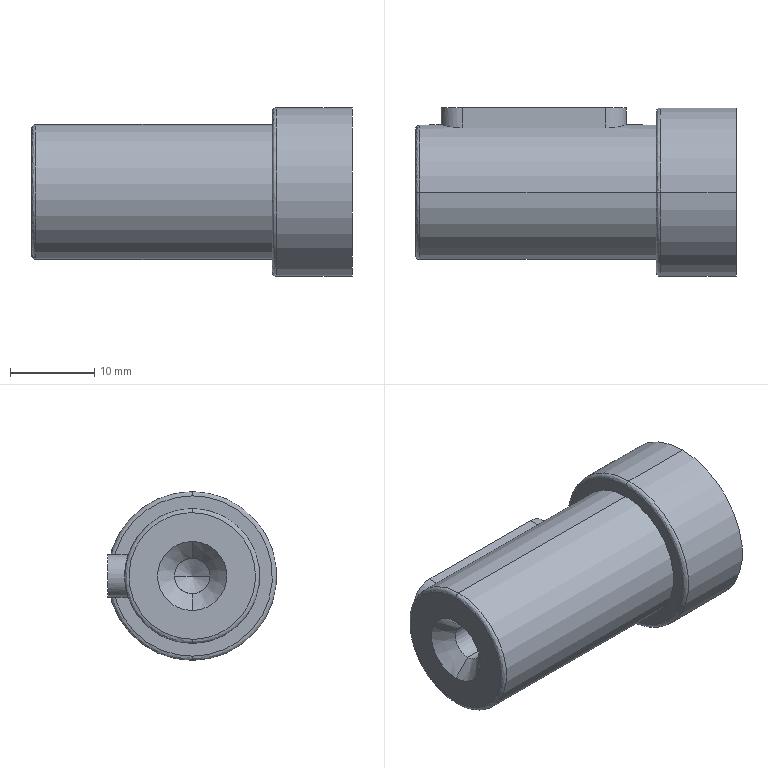Part | STEP file | _X2_8f9351fa884c661f67b6_X0_MAB060-16X28.5XM5_2.STEP.STEP | 1 solid | 22 faces | box 38 x 20 x 20 mm | volume 8651 mm3 | cylinder 8 | plane 6 | spline 4 | cone 4 | commonest cylinder face diameters 4.2 x2 5 x2 16 x2 20 x2
STEP:
#1=CARTESIAN_POINT('',(9.288,0.,7.5));
#2=VERTEX_POINT('',#1);
#3=CARTESIAN_POINT('',(9.288,0.,-7.5));
#4=VERTEX_POINT('',#3);
#5=CARTESIAN_POINT('',(9.288,0.,7.5));
#6=CARTESIAN_POINT('',(9.288,-15.,7.5));
#7=CARTESIAN_POINT('',(9.288,-15.,-7.5));
#8=CARTESIAN_POINT('',(9.288,0.,-7.5));
#9=(BOUNDED_CURVE()B_SPLINE_CURVE(3,(#5,#6,#7,#8),.UNSPECIFIED.,.F.,.F.)B_SPLINE_CURVE_WITH_KNOTS((4,4),(0.,1.),.UNSPECIFIED.)CURVE()GEOMETRIC_REPRESENTATION_ITEM()RATIONAL_B_SPLINE_CURVE((1.,0.3333,0.3333,1.))REPRESENTATION_ITEM(''));
#10=EDGE_CURVE('',#2,#4,#9,.T.);
#11=ORIENTED_EDGE('',*,*,#10,.T.);
#12=CARTESIAN_POINT('',(9.788,0.,-8.));
#13=VERTEX_POINT('',#12);
#14=CARTESIAN_POINT('',(9.788,0.,-7.5));
#15=DIRECTION('',(0.,-1.,0.));
#16=DIRECTION('',(0.,0.,-1.));
#17=AXIS2_PLACEMENT_3D('',#14,#15,#16);
#18=CIRCLE('',#17,0.5);
#19=EDGE_CURVE('',#4,#13,#18,.T.);
#20=ORIENTED_EDGE('',*,*,#19,.T.);
#21=CARTESIAN_POINT('',(9.788,0.,8.));
#22=VERTEX_POINT('',#21);
#23=CARTESIAN_POINT('',(9.788,0.,0.));
#24=DIRECTION('',(1.,0.,0.));
#25=DIRECTION('',(0.,0.,-1.));
#26=AXIS2_PLACEMENT_3D('',#23,#24,#25);
#27=CIRCLE('',#26,8.);
#28=EDGE_CURVE('',#22,#13,#27,.T.);
#29=ORIENTED_EDGE('',*,*,#28,.F.);
#30=CARTESIAN_POINT('',(9.788,0.,7.5));
#31=DIRECTION('',(0.,1.,0.));
#32=DIRECTION('',(0.,0.,1.));
#33=AXIS2_PLACEMENT_3D('',#30,#31,#32);
#34=CIRCLE('',#33,0.5);
#35=EDGE_CURVE('',#2,#22,#34,.T.);
#36=ORIENTED_EDGE('',*,*,#35,.F.);
#37=EDGE_LOOP('',(#11,#20,#29,#36));
#38=FACE_OUTER_BOUND('',#37,.T.);
#39=CARTESIAN_POINT('',(9.288,0.,-7.5));
#40=CARTESIAN_POINT('',(9.288,-15.,-7.5));
#41=CARTESIAN_POINT('',(9.288,-15.,7.5));
#42=CARTESIAN_POINT('',(9.288,0.,7.5));
#43=CARTESIAN_POINT('',(9.288,0.,-7.793));
#44=CARTESIAN_POINT('',(9.288,-15.586,-7.793));
#45=CARTESIAN_POINT('',(9.288,-15.586,7.793));
#46=CARTESIAN_POINT('',(9.288,0.,7.793));
#47=CARTESIAN_POINT('',(9.495,0.,-8.));
#48=CARTESIAN_POINT('',(9.495,-16.,-8.));
#49=CARTESIAN_POINT('',(9.495,-16.,8.));
#50=CARTESIAN_POINT('',(9.495,0.,8.));
#51=CARTESIAN_POINT('',(9.788,0.,-8.));
#52=CARTESIAN_POINT('',(9.788,-16.,-8.));
#53=CARTESIAN_POINT('',(9.788,-16.,8.));
#54=CARTESIAN_POINT('',(9.788,0.,8.));
#55=(BOUNDED_SURFACE()B_SPLINE_SURFACE(3,3,((#39,#40,#41,#42),(#43,#44,#45,#46),(#47,#48,#49,#50),(#51,#52,#53,#54)),.UNSPECIFIED.,.F.,.F.,.T.)B_SPLINE_SURFACE_WITH_KNOTS((4,4),(4,4),(0.,1.),(0.,1.),.UNSPECIFIED.)GEOMETRIC_REPRESENTATION_ITEM()RATIONAL_B_SPLINE_SURFACE(((1.,0.3333,0.3333,1.),(0.8047,0.2682,0.2682,0.8047),(0.8047,0.2682,0.2682,0.8047),(1.,0.3333,0.3333,1.)))REPRESENTATION_ITEM('')SURFACE());
#56=ADVANCED_FACE('',(#38),#55,.T.);
#57=CARTESIAN_POINT('',(37.788,0.,-9.5));
#58=VERTEX_POINT('',#57);
#59=CARTESIAN_POINT('',(37.788,0.,9.5));
#60=VERTEX_POINT('',#59);
#61=CARTESIAN_POINT('',(37.788,0.,-9.5));
#62=CARTESIAN_POINT('',(37.788,-0.2904,-9.5));
#63=CARTESIAN_POINT('',(37.788,-0.7244,-9.48));
#64=CARTESIAN_POINT('',(37.788,-1.228,-9.422));
#65=CARTESIAN_POINT('',(37.788,-1.478,-9.385));
#66=CARTESIAN_POINT('',(37.788,-1.586,-9.367));
#67=CARTESIAN_POINT('',(37.788,-1.657,-9.354));
#68=CARTESIAN_POINT('',(37.788,-1.691,-9.348));
#69=CARTESIAN_POINT('',(37.788,-2.031,-9.285));
#70=CARTESIAN_POINT('',(37.788,-2.48,-9.18));
#71=CARTESIAN_POINT('',(37.788,-2.992,-9.019));
#72=CARTESIAN_POINT('',(37.788,-3.245,-8.929));
#73=CARTESIAN_POINT('',(37.788,-3.353,-8.889));
#74=CARTESIAN_POINT('',(37.788,-3.425,-8.861));
#75=CARTESIAN_POINT('',(37.788,-3.46,-8.848));
#76=CARTESIAN_POINT('',(37.788,-3.795,-8.715));
#77=CARTESIAN_POINT('',(37.788,-4.232,-8.516));
#78=CARTESIAN_POINT('',(37.788,-4.722,-8.246));
#79=CARTESIAN_POINT('',(37.788,-4.927,-8.123));
#80=CARTESIAN_POINT('',(37.788,-5.064,-8.038));
#81=CARTESIAN_POINT('',(37.788,-5.13,-7.996));
#82=CARTESIAN_POINT('',(37.788,-5.747,-7.593));
#83=CARTESIAN_POINT('',(37.788,-6.254,-7.181));
#84=CARTESIAN_POINT('',(37.788,-6.949,-6.486));
#85=CARTESIAN_POINT('',(37.788,-7.277,-6.122));
#86=CARTESIAN_POINT('',(37.788,-7.626,-5.67));
#87=CARTESIAN_POINT('',(37.788,-7.768,-5.47));
#88=CARTESIAN_POINT('',(37.788,-7.861,-5.335));
#89=CARTESIAN_POINT('',(37.788,-7.908,-5.266));
#90=CARTESIAN_POINT('',(37.788,-8.127,-4.93));
#91=CARTESIAN_POINT('',(37.788,-8.369,-4.516));
#92=CARTESIAN_POINT('',(37.788,-8.614,-4.013));
#93=CARTESIAN_POINT('',(37.788,-8.726,-3.757));
#94=CARTESIAN_POINT('',(37.788,-8.773,-3.646));
#95=CARTESIAN_POINT('',(37.788,-8.803,-3.571));
#96=CARTESIAN_POINT('',(37.788,-8.819,-3.533));
#97=CARTESIAN_POINT('',(37.788,-8.946,-3.211));
#98=CARTESIAN_POINT('',(37.788,-9.095,-2.775));
#99=CARTESIAN_POINT('',(37.788,-9.231,-2.255));
#100=CARTESIAN_POINT('',(37.788,-9.289,-1.993));
#101=CARTESIAN_POINT('',(37.788,-9.312,-1.88));
#102=CARTESIAN_POINT('',(37.788,-9.327,-1.804));
#103=CARTESIAN_POINT('',(37.788,-9.335,-1.764));
#104=CARTESIAN_POINT('',(37.788,-9.447,-1.158));
#105=CARTESIAN_POINT('',(37.788,-9.5,-0.5807));
#106=CARTESIAN_POINT('',(37.788,-9.5,0.2904));
#107=CARTESIAN_POINT('',(37.788,-9.48,0.7242));
#108=CARTESIAN_POINT('',(37.788,-9.422,1.227));
#109=CARTESIAN_POINT('',(37.788,-9.385,1.478));
#110=CARTESIAN_POINT('',(37.788,-9.367,1.586));
#111=CARTESIAN_POINT('',(37.788,-9.354,1.657));
#112=CARTESIAN_POINT('',(37.788,-9.348,1.691));
#113=CARTESIAN_POINT('',(37.788,-9.285,2.031));
#114=CARTESIAN_POINT('',(37.788,-9.18,2.48));
#115=CARTESIAN_POINT('',(37.788,-9.019,2.992));
#116=CARTESIAN_POINT('',(37.788,-8.929,3.245));
#117=CARTESIAN_POINT('',(37.788,-8.889,3.353));
#118=CARTESIAN_POINT('',(37.788,-8.861,3.425));
#119=CARTESIAN_POINT('',(37.788,-8.848,3.46));
#120=CARTESIAN_POINT('',(37.788,-8.715,3.795));
#121=CARTESIAN_POINT('',(37.788,-8.516,4.232));
#122=CARTESIAN_POINT('',(37.788,-8.246,4.722));
#123=CARTESIAN_POINT('',(37.788,-8.123,4.927));
#124=CARTESIAN_POINT('',(37.788,-8.038,5.064));
#125=CARTESIAN_POINT('',(37.788,-7.996,5.13));
#126=CARTESIAN_POINT('',(37.788,-7.593,5.747));
#127=CARTESIAN_POINT('',(37.788,-7.181,6.254));
#128=CARTESIAN_POINT('',(37.788,-6.486,6.949));
#129=CARTESIAN_POINT('',(37.788,-6.122,7.277));
#130=CARTESIAN_POINT('',(37.788,-5.67,7.626));
#131=CARTESIAN_POINT('',(37.788,-5.47,7.768));
#132=CARTESIAN_POINT('',(37.788,-5.335,7.861));
#133=CARTESIAN_POINT('',(37.788,-5.266,7.908));
#134=CARTESIAN_POINT('',(37.788,-4.93,8.127));
#135=CARTESIAN_POINT('',(37.788,-4.516,8.369));
#136=CARTESIAN_POINT('',(37.788,-4.013,8.614));
#137=CARTESIAN_POINT('',(37.788,-3.757,8.726));
#138=CARTESIAN_POINT('',(37.788,-3.646,8.773));
#139=CARTESIAN_POINT('',(37.788,-3.571,8.803));
#140=CARTESIAN_POINT('',(37.788,-3.533,8.819));
#141=CARTESIAN_POINT('',(37.788,-3.211,8.946));
#142=CARTESIAN_POINT('',(37.788,-2.775,9.095));
#143=CARTESIAN_POINT('',(37.788,-2.255,9.231));
#144=CARTESIAN_POINT('',(37.788,-1.993,9.289));
#145=CARTESIAN_POINT('',(37.788,-1.88,9.312));
#146=CARTESIAN_POINT('',(37.788,-1.804,9.327));
#147=CARTESIAN_POINT('',(37.788,-1.764,9.335));
#148=CARTESIAN_POINT('',(37.788,-1.157,9.447));
#149=CARTESIAN_POINT('',(37.788,-0.5812,9.5));
#150=CARTESIAN_POINT('',(37.788,0.,9.5));
#151=B_SPLINE_CURVE_WITH_KNOTS('',3,(#61,#62,#63,#64,#65,#66,#67,#68,#69,#70,#71,#72,#73,#74,#75,#76,#77,#78,#79,#80,#81,#82,#83,#84,#85,#86,#87,#88,#89,#90,#91,#92,#93,#94,#95,#96,#97,#98,#99,#100,#101,#102,#103,#104,#105,#106,#107,#108,#109,#110,#111,#112,#113,#114,#115,#116,#117,#118,#119,#120,#121,#122,#123,#124,#125,#126,#127,#128,#129,#130,#131,#132,#133,#134,#135,#136,#137,#138,#139,#140,#141,#142,#143,#144,#145,#146,#147,#148,#149,#150),.UNSPECIFIED.,.F.,.F.,(4,1,1,1,2,2,1,1,1,2,2,1,1,2,2,2,1,1,2,2,1,1,1,2,2,1,1,1,2,2,2,1,1,1,2,2,1,1,1,2,2,1,1,2,2,2,1,1,2,2,1,1,1,2,2,1,1,1,2,2,4),(0.,0.03125,0.04688,0.05469,0.05859,0.0625,0.09375,0.1094,0.1172,0.1211,0.125,0.1563,0.1719,0.1797,0.1875,0.25,0.2813,0.2969,0.3047,0.3125,0.3438,0.3594,0.3672,0.3711,0.375,0.4063,0.4219,0.4297,0.4336,0.4375,0.5,0.5313,0.5469,0.5547,0.5586,0.5625,0.5938,0.6094,0.6172,0.6211,0.625,0.6563,0.6719,0.6797,0.6875,0.75,0.7813,0.7969,0.8047,0.8125,0.8438,0.8594,0.8672,0.8711,0.875,0.9063,0.9219,0.9297,0.9336,0.9375,1.),.UNSPECIFIED.);
#152=EDGE_CURVE('',#58,#60,#151,.T.);
#153=ORIENTED_EDGE('',*,*,#152,.F.);
#154=CARTESIAN_POINT('',(38.288,0.,-10.));
#155=VERTEX_POINT('',#154);
#156=CARTESIAN_POINT('',(38.288,0.,-9.5));
#157=DIRECTION('',(0.,-1.,0.));
#158=DIRECTION('',(0.,0.,-1.));
#159=AXIS2_PLACEMENT_3D('',#156,#157,#158);
#160=CIRCLE('',#159,0.5);
#161=EDGE_CURVE('',#58,#155,#160,.T.);
#162=ORIENTED_EDGE('',*,*,#161,.T.);
#163=CARTESIAN_POINT('',(38.288,0.,10.));
#164=VERTEX_POINT('',#163);
#165=CARTESIAN_POINT('',(38.288,0.,0.));
#166=DIRECTION('',(-1.,0.,0.));
#167=DIRECTION('',(0.,0.,1.));
#168=AXIS2_PLACEMENT_3D('',#165,#166,#167);
#169=CIRCLE('',#168,10.);
#170=EDGE_CURVE('',#155,#164,#169,.T.);
#171=ORIENTED_EDGE('',*,*,#170,.T.);
#172=CARTESIAN_POINT('',(38.288,0.,9.5));
#173=DIRECTION('',(0.,1.,0.));
#174=DIRECTION('',(0.,0.,1.));
#175=AXIS2_PLACEMENT_3D('',#172,#173,#174);
#176=CIRCLE('',#175,0.5);
#177=EDGE_CURVE('',#60,#164,#176,.T.);
#178=ORIENTED_EDGE('',*,*,#177,.F.);
#179=EDGE_LOOP('',(#153,#162,#171,#178));
#180=FACE_OUTER_BOUND('',#179,.T.);
#181=CARTESIAN_POINT('',(37.788,0.,-9.5));
#182=CARTESIAN_POINT('',(37.788,-19.,-9.5));
#183=CARTESIAN_POINT('',(37.788,-19.,9.5));
#184=CARTESIAN_POINT('',(37.788,0.,9.5));
#185=CARTESIAN_POINT('',(37.788,0.,-9.793));
#186=CARTESIAN_POINT('',(37.788,-19.586,-9.793));
#187=CARTESIAN_POINT('',(37.788,-19.586,9.793));
#188=CARTESIAN_POINT('',(37.788,0.,9.793));
#189=CARTESIAN_POINT('',(37.995,0.,-10.));
#190=CARTESIAN_POINT('',(37.995,-20.,-10.));
#191=CARTESIAN_POINT('',(37.995,-20.,10.));
#192=CARTESIAN_POINT('',(37.995,0.,10.));
#193=CARTESIAN_POINT('',(38.288,0.,-10.));
#194=CARTESIAN_POINT('',(38.288,-20.,-10.));
#195=CARTESIAN_POINT('',(38.288,-20.,10.));
#196=CARTESIAN_POINT('',(38.288,0.,10.));
#197=(BOUNDED_SURFACE()B_SPLINE_SURFACE(3,3,((#181,#182,#183,#184),(#185,#186,#187,#188),(#189,#190,#191,#192),(#193,#194,#195,#196)),.UNSPECIFIED.,.F.,.F.,.F.)B_SPLINE_SURFACE_WITH_KNOTS((4,4),(4,4),(0.,1.),(0.,1.),.UNSPECIFIED.)GEOMETRIC_REPRESENTATION_ITEM()RATIONAL_B_SPLINE_SURFACE(((1.,0.3333,0.3333,1.),(0.8047,0.2682,0.2682,0.8047),(0.8047,0.2682,0.2682,0.8047),(1.,0.3333,0.3333,1.)))REPRESENTATION_ITEM('')SURFACE());
#198=ADVANCED_FACE('',(#180),#197,.T.);
#199=CARTESIAN_POINT('',(31.788,7.599,-2.5));
#200=VERTEX_POINT('',#199);
#201=CARTESIAN_POINT('',(31.788,7.599,2.5));
#202=VERTEX_POINT('',#201);
#203=CARTESIAN_POINT('',(31.788,7.599,-2.5));
#204=CARTESIAN_POINT('',(31.954,7.599,-2.5));
#205=CARTESIAN_POINT('',(32.117,7.605,-2.484));
#206=CARTESIAN_POINT('',(32.438,7.625,-2.419));
#207=CARTESIAN_POINT('',(32.597,7.641,-2.371));
#208=CARTESIAN_POINT('',(32.899,7.679,-2.245));
#209=CARTESIAN_POINT('',(33.042,7.701,-2.168));
#210=CARTESIAN_POINT('',(33.313,7.75,-1.987));
#211=CARTESIAN_POINT('',(33.441,7.776,-1.882));
#212=CARTESIAN_POINT('',(33.784,7.854,-1.539));
#213=CARTESIAN_POINT('',(33.97,7.906,-1.262));
#214=CARTESIAN_POINT('',(34.158,7.96,-0.8114));
#215=CARTESIAN_POINT('',(34.206,7.975,-0.6527));
#216=CARTESIAN_POINT('',(34.271,7.995,-0.3296));
#217=CARTESIAN_POINT('',(34.287,8.,-0.1667));
#218=CARTESIAN_POINT('',(34.288,8.,0.1617));
#219=CARTESIAN_POINT('',(34.271,7.995,0.3285));
#220=CARTESIAN_POINT('',(34.207,7.975,0.6499));
#221=CARTESIAN_POINT('',(34.16,7.961,0.8063));
#222=CARTESIAN_POINT('',(34.033,7.924,1.11));
#223=CARTESIAN_POINT('',(33.956,7.902,1.255));
#224=CARTESIAN_POINT('',(33.775,7.855,1.525));
#225=CARTESIAN_POINT('',(33.671,7.828,1.652));
#226=CARTESIAN_POINT('',(33.441,7.776,1.883));
#227=CARTESIAN_POINT('',(33.316,7.75,1.985));
#228=CARTESIAN_POINT('',(33.046,7.702,2.166));
#229=CARTESIAN_POINT('',(32.9,7.679,2.245));
#230=CARTESIAN_POINT('',(32.599,7.641,2.37));
#231=CARTESIAN_POINT('',(32.443,7.626,2.418));
#232=CARTESIAN_POINT('',(32.12,7.605,2.483));
#233=CARTESIAN_POINT('',(31.954,7.599,2.5));
#234=CARTESIAN_POINT('',(31.788,7.599,2.5));
#235=B_SPLINE_CURVE_WITH_KNOTS('',3,(#203,#204,#205,#206,#207,#208,#209,#210,#211,#212,#213,#214,#215,#216,#217,#218,#219,#220,#221,#222,#223,#224,#225,#226,#227,#228,#229,#230,#231,#232,#233,#234),.UNSPECIFIED.,.F.,.F.,(4,2,2,2,2,2,2,2,2,2,2,2,2,2,2,4),(0.,0.0004914,0.0009828,0.001474,0.001966,0.002949,0.00344,0.003931,0.004423,0.004914,0.005406,0.005897,0.006388,0.00688,0.007371,0.007863),.UNSPECIFIED.);
#236=EDGE_CURVE('',#200,#202,#235,.T.);
#237=ORIENTED_EDGE('',*,*,#236,.T.);
#238=CARTESIAN_POINT('',(14.788,7.599,2.5));
#239=VERTEX_POINT('',#238);
#240=CARTESIAN_POINT('',(-25.212,7.599,2.5));
#241=DIRECTION('',(-1.,0.,0.));
#242=VECTOR('',#241,1000.);
#243=LINE('',#240,#242);
#244=EDGE_CURVE('',#202,#239,#243,.T.);
#245=ORIENTED_EDGE('',*,*,#244,.T.);
#246=CARTESIAN_POINT('',(14.788,7.599,-2.5));
#247=VERTEX_POINT('',#246);
#248=CARTESIAN_POINT('',(14.788,7.599,2.5));
#249=CARTESIAN_POINT('',(14.621,7.599,2.5));
#250=CARTESIAN_POINT('',(14.458,7.605,2.484));
#251=CARTESIAN_POINT('',(14.137,7.625,2.419));
#252=CARTESIAN_POINT('',(13.978,7.641,2.371));
#253=CARTESIAN_POINT('',(13.676,7.679,2.245));
#254=CARTESIAN_POINT('',(13.533,7.701,2.168));
#255=CARTESIAN_POINT('',(13.262,7.75,1.987));
#256=CARTESIAN_POINT('',(13.134,7.776,1.882));
#257=CARTESIAN_POINT('',(12.791,7.854,1.539));
#258=CARTESIAN_POINT('',(12.605,7.906,1.262));
#259=CARTESIAN_POINT('',(12.417,7.96,0.8114));
#260=CARTESIAN_POINT('',(12.369,7.975,0.6527));
#261=CARTESIAN_POINT('',(12.304,7.995,0.3296));
#262=CARTESIAN_POINT('',(12.288,8.,0.1667));
#263=CARTESIAN_POINT('',(12.287,8.,-0.1617));
#264=CARTESIAN_POINT('',(12.304,7.995,-0.3285));
#265=CARTESIAN_POINT('',(12.368,7.975,-0.6499));
#266=CARTESIAN_POINT('',(12.415,7.961,-0.8063));
#267=CARTESIAN_POINT('',(12.542,7.924,-1.11));
#268=CARTESIAN_POINT('',(12.619,7.902,-1.255));
#269=CARTESIAN_POINT('',(12.8,7.855,-1.525));
#270=CARTESIAN_POINT('',(12.904,7.828,-1.652));
#271=CARTESIAN_POINT('',(13.134,7.776,-1.883));
#272=CARTESIAN_POINT('',(13.26,7.75,-1.985));
#273=CARTESIAN_POINT('',(13.529,7.702,-2.166));
#274=CARTESIAN_POINT('',(13.675,7.679,-2.245));
#275=CARTESIAN_POINT('',(13.976,7.641,-2.37));
#276=CARTESIAN_POINT('',(14.132,7.626,-2.418));
#277=CARTESIAN_POINT('',(14.455,7.605,-2.483));
#278=CARTESIAN_POINT('',(14.621,7.599,-2.5));
#279=CARTESIAN_POINT('',(14.788,7.599,-2.5));
#280=B_SPLINE_CURVE_WITH_KNOTS('',3,(#248,#249,#250,#251,#252,#253,#254,#255,#256,#257,#258,#259,#260,#261,#262,#263,#264,#265,#266,#267,#268,#269,#270,#271,#272,#273,#274,#275,#276,#277,#278,#279),.UNSPECIFIED.,.F.,.F.,(4,2,2,2,2,2,2,2,2,2,2,2,2,2,2,4),(0.,0.0004914,0.0009828,0.001474,0.001966,0.002949,0.00344,0.003931,0.004423,0.004914,0.005406,0.005897,0.006388,0.00688,0.007371,0.007863),.UNSPECIFIED.);
#281=EDGE_CURVE('',#239,#247,#280,.T.);
#282=ORIENTED_EDGE('',*,*,#281,.T.);
#283=CARTESIAN_POINT('',(-25.212,7.599,-2.5));
#284=DIRECTION('',(1.,0.,0.));
#285=VECTOR('',#284,1000.);
#286=LINE('',#283,#285);
#287=EDGE_CURVE('',#247,#200,#286,.T.);
#288=ORIENTED_EDGE('',*,*,#287,.T.);
#289=EDGE_LOOP('',(#237,#245,#282,#288));
#290=FACE_BOUND('',#289,.T.);
#291=CARTESIAN_POINT('',(9.788,0.,0.));
#292=DIRECTION('',(1.,0.,0.));
#293=DIRECTION('',(0.,0.,-1.));
#294=AXIS2_PLACEMENT_3D('',#291,#292,#293);
#295=CIRCLE('',#294,8.);
#296=EDGE_CURVE('',#13,#22,#295,.T.);
#297=ORIENTED_EDGE('',*,*,#296,.T.);
#298=CARTESIAN_POINT('',(37.788,0.,8.));
#299=VERTEX_POINT('',#298);
#300=CARTESIAN_POINT('',(-25.212,0.,8.));
#301=DIRECTION('',(1.,0.,0.));
#302=VECTOR('',#301,1000.);
#303=LINE('',#300,#302);
#304=EDGE_CURVE('',#22,#299,#303,.T.);
#305=ORIENTED_EDGE('',*,*,#304,.T.);
#306=CARTESIAN_POINT('',(37.788,0.,-8.));
#307=VERTEX_POINT('',#306);
#308=CARTESIAN_POINT('',(37.788,0.,0.));
#309=DIRECTION('',(-1.,0.,0.));
#310=DIRECTION('',(0.,0.,-1.));
#311=AXIS2_PLACEMENT_3D('',#308,#309,#310);
#312=CIRCLE('',#311,8.);
#313=EDGE_CURVE('',#299,#307,#312,.T.);
#314=ORIENTED_EDGE('',*,*,#313,.T.);
#315=CARTESIAN_POINT('',(-25.212,0.,-8.));
#316=DIRECTION('',(1.,0.,0.));
#317=VECTOR('',#316,1000.);
#318=LINE('',#315,#317);
#319=EDGE_CURVE('',#13,#307,#318,.T.);
#320=ORIENTED_EDGE('',*,*,#319,.F.);
#321=EDGE_LOOP('',(#297,#305,#314,#320));
#322=FACE_OUTER_BOUND('',#321,.T.);
#323=CARTESIAN_POINT('',(-25.212,0.,0.));
#324=DIRECTION('',(1.,0.,0.));
#325=DIRECTION('',(0.,0.,-1.));
#326=AXIS2_PLACEMENT_3D('',#323,#324,#325);
#327=CYLINDRICAL_SURFACE('',#326,8.);
#328=ADVANCED_FACE('',(#290,#322),#327,.T.);
#329=CARTESIAN_POINT('',(47.288,0.,10.));
#330=VERTEX_POINT('',#329);
#331=CARTESIAN_POINT('',(47.288,0.,-10.));
#332=VERTEX_POINT('',#331);
#333=CARTESIAN_POINT('',(47.288,0.,0.));
#334=DIRECTION('',(-1.,0.,0.));
#335=DIRECTION('',(0.,0.,1.));
#336=AXIS2_PLACEMENT_3D('',#333,#334,#335);
#337=CIRCLE('',#336,10.);
#338=EDGE_CURVE('',#330,#332,#337,.T.);
#339=ORIENTED_EDGE('',*,*,#338,.T.);
#340=CARTESIAN_POINT('',(-19.212,0.,-10.));
#341=DIRECTION('',(-1.,0.,0.));
#342=VECTOR('',#341,1000.);
#343=LINE('',#340,#342);
#344=EDGE_CURVE('',#332,#155,#343,.T.);
#345=ORIENTED_EDGE('',*,*,#344,.T.);
#346=CARTESIAN_POINT('',(38.288,0.,0.));
#347=DIRECTION('',(-1.,0.,0.));
#348=DIRECTION('',(0.,0.,1.));
#349=AXIS2_PLACEMENT_3D('',#346,#347,#348);
#350=CIRCLE('',#349,10.);
#351=EDGE_CURVE('',#164,#155,#350,.T.);
#352=ORIENTED_EDGE('',*,*,#351,.F.);
#353=CARTESIAN_POINT('',(-19.212,0.,10.));
#354=DIRECTION('',(-1.,0.,0.));
#355=VECTOR('',#354,1000.);
#356=LINE('',#353,#355);
#357=EDGE_CURVE('',#330,#164,#356,.T.);
#358=ORIENTED_EDGE('',*,*,#357,.F.);
#359=EDGE_LOOP('',(#339,#345,#352,#358));
#360=FACE_OUTER_BOUND('',#359,.T.);
#361=CARTESIAN_POINT('',(-19.212,0.,0.));
#362=DIRECTION('',(-1.,0.,0.));
#363=DIRECTION('',(0.,0.,1.));
#364=AXIS2_PLACEMENT_3D('',#361,#362,#363);
#365=CYLINDRICAL_SURFACE('',#364,10.);
#366=ADVANCED_FACE('',(#360),#365,.T.);
#367=CARTESIAN_POINT('',(11.288,0.,-2.1));
#368=VERTEX_POINT('',#367);
#369=CARTESIAN_POINT('',(11.288,0.,2.1));
#370=VERTEX_POINT('',#369);
#371=CARTESIAN_POINT('',(11.288,0.,0.));
#372=DIRECTION('',(-1.,0.,0.));
#373=DIRECTION('',(0.,0.,1.));
#374=AXIS2_PLACEMENT_3D('',#371,#372,#373);
#375=CIRCLE('',#374,2.1);
#376=EDGE_CURVE('',#368,#370,#375,.T.);
#377=ORIENTED_EDGE('',*,*,#376,.F.);
#378=CARTESIAN_POINT('',(9.288,0.,-4.1));
#379=VERTEX_POINT('',#378);
#380=CARTESIAN_POINT('',(9.288,0.,-4.1));
#381=DIRECTION('',(-0.7071,0.,-0.7071));
#382=VECTOR('',#381,1000.);
#383=LINE('',#380,#382);
#384=EDGE_CURVE('',#368,#379,#383,.T.);
#385=ORIENTED_EDGE('',*,*,#384,.T.);
#386=CARTESIAN_POINT('',(9.288,0.,4.1));
#387=VERTEX_POINT('',#386);
#388=CARTESIAN_POINT('',(9.288,0.,0.));
#389=DIRECTION('',(1.,0.,0.));
#390=DIRECTION('',(0.,0.,1.));
#391=AXIS2_PLACEMENT_3D('',#388,#389,#390);
#392=CIRCLE('',#391,4.1);
#393=EDGE_CURVE('',#387,#379,#392,.T.);
#394=ORIENTED_EDGE('',*,*,#393,.F.);
#395=CARTESIAN_POINT('',(9.288,0.,4.1));
#396=DIRECTION('',(-0.7071,0.,0.7071));
#397=VECTOR('',#396,1000.);
#398=LINE('',#395,#397);
#399=EDGE_CURVE('',#370,#387,#398,.T.);
#400=ORIENTED_EDGE('',*,*,#399,.F.);
#401=EDGE_LOOP('',(#377,#385,#394,#400));
#402=FACE_OUTER_BOUND('',#401,.T.);
#403=CARTESIAN_POINT('',(9.288,0.,0.));
#404=DIRECTION('',(-1.,0.,0.));
#405=DIRECTION('',(0.,0.,1.));
#406=AXIS2_PLACEMENT_3D('',#403,#404,#405);
#407=CONICAL_SURFACE('',#406,4.1,0.7854);
#408=ADVANCED_FACE('',(#402),#407,.F.);
#409=CARTESIAN_POINT('',(26.688,0.,-2.1));
#410=VERTEX_POINT('',#409);
#411=CARTESIAN_POINT('',(26.688,-2.1,0.));
#412=VERTEX_POINT('',#411);
#413=CARTESIAN_POINT('',(26.688,0.,0.));
#414=DIRECTION('',(-1.,0.,0.));
#415=DIRECTION('',(0.,0.,1.));
#416=AXIS2_PLACEMENT_3D('',#413,#414,#415);
#417=CIRCLE('',#416,2.1);
#418=EDGE_CURVE('',#410,#412,#417,.T.);
#419=ORIENTED_EDGE('',*,*,#418,.F.);
#420=CARTESIAN_POINT('',(9.288,0.,-2.1));
#421=DIRECTION('',(-1.,0.,0.));
#422=VECTOR('',#421,1000.);
#423=LINE('',#420,#422);
#424=EDGE_CURVE('',#410,#368,#423,.T.);
#425=ORIENTED_EDGE('',*,*,#424,.T.);
#426=ORIENTED_EDGE('',*,*,#376,.T.);
#427=CARTESIAN_POINT('',(26.688,0.,2.1));
#428=VERTEX_POINT('',#427);
#429=CARTESIAN_POINT('',(9.288,0.,2.1));
#430=DIRECTION('',(-1.,0.,0.));
#431=VECTOR('',#430,1000.);
#432=LINE('',#429,#431);
#433=EDGE_CURVE('',#428,#370,#432,.T.);
#434=ORIENTED_EDGE('',*,*,#433,.F.);
#435=CARTESIAN_POINT('',(26.688,0.,0.));
#436=DIRECTION('',(-1.,0.,0.));
#437=DIRECTION('',(0.,0.,1.));
#438=AXIS2_PLACEMENT_3D('',#435,#436,#437);
#439=CIRCLE('',#438,2.1);
#440=EDGE_CURVE('',#412,#428,#439,.T.);
#441=ORIENTED_EDGE('',*,*,#440,.F.);
#442=EDGE_LOOP('',(#419,#425,#426,#434,#441));
#443=FACE_OUTER_BOUND('',#442,.T.);
#444=CARTESIAN_POINT('',(9.288,0.,0.));
#445=DIRECTION('',(-1.,0.,0.));
#446=DIRECTION('',(0.,0.,1.));
#447=AXIS2_PLACEMENT_3D('',#444,#445,#446);
#448=CYLINDRICAL_SURFACE('',#447,2.1);
#449=ADVANCED_FACE('',(#443),#448,.F.);
#450=CARTESIAN_POINT('',(27.949,0.,0.));
#451=VERTEX_POINT('',#450);
#452=CARTESIAN_POINT('',(26.688,-2.1,0.));
#453=DIRECTION('',(-0.515,-0.8572,0.));
#454=VECTOR('',#453,1000.);
#455=LINE('',#452,#454);
#456=EDGE_CURVE('',#451,#412,#455,.T.);
#457=ORIENTED_EDGE('',*,*,#456,.F.);
#458=CARTESIAN_POINT('',(26.688,2.1,0.));
#459=VERTEX_POINT('',#458);
#460=CARTESIAN_POINT('',(26.688,2.1,0.));
#461=DIRECTION('',(-0.515,0.8572,0.));
#462=VECTOR('',#461,1000.);
#463=LINE('',#460,#462);
#464=EDGE_CURVE('',#451,#459,#463,.T.);
#465=ORIENTED_EDGE('',*,*,#464,.T.);
#466=CARTESIAN_POINT('',(26.688,0.,0.));
#467=DIRECTION('',(-1.,0.,0.));
#468=DIRECTION('',(0.,0.,1.));
#469=AXIS2_PLACEMENT_3D('',#466,#467,#468);
#470=CIRCLE('',#469,2.1);
#471=EDGE_CURVE('',#459,#410,#470,.T.);
#472=ORIENTED_EDGE('',*,*,#471,.T.);
#473=ORIENTED_EDGE('',*,*,#418,.T.);
#474=EDGE_LOOP('',(#457,#465,#472,#473));
#475=FACE_OUTER_BOUND('',#474,.T.);
#476=CARTESIAN_POINT('',(26.688,0.,0.));
#477=DIRECTION('',(-1.,0.,0.));
#478=DIRECTION('',(0.,-1.,0.));
#479=AXIS2_PLACEMENT_3D('',#476,#477,#478);
#480=CONICAL_SURFACE('',#479,2.1,1.03);
#481=ADVANCED_FACE('',(#475),#480,.F.);
#482=ORIENTED_EDGE('',*,*,#304,.F.);
#483=ORIENTED_EDGE('',*,*,#28,.T.);
#484=ORIENTED_EDGE('',*,*,#319,.T.);
#485=CARTESIAN_POINT('',(37.788,0.,0.));
#486=DIRECTION('',(-1.,0.,0.));
#487=DIRECTION('',(0.,0.,-1.));
#488=AXIS2_PLACEMENT_3D('',#485,#486,#487);
#489=CIRCLE('',#488,8.);
#490=EDGE_CURVE('',#307,#299,#489,.T.);
#491=ORIENTED_EDGE('',*,*,#490,.T.);
#492=EDGE_LOOP('',(#482,#483,#484,#491));
#493=FACE_OUTER_BOUND('',#492,.T.);
#494=CARTESIAN_POINT('',(-25.212,0.,0.));
#495=DIRECTION('',(1.,0.,0.));
#496=DIRECTION('',(0.,0.,-1.));
#497=AXIS2_PLACEMENT_3D('',#494,#495,#496);
#498=CYLINDRICAL_SURFACE('',#497,8.);
#499=ADVANCED_FACE('',(#493),#498,.T.);
#500=CARTESIAN_POINT('',(37.788,0.,9.5));
#501=CARTESIAN_POINT('',(37.788,0.2904,9.5));
#502=CARTESIAN_POINT('',(37.788,0.7244,9.48));
#503=CARTESIAN_POINT('',(37.788,1.228,9.422));
#504=CARTESIAN_POINT('',(37.788,1.478,9.385));
#505=CARTESIAN_POINT('',(37.788,1.586,9.367));
#506=CARTESIAN_POINT('',(37.788,1.657,9.354));
#507=CARTESIAN_POINT('',(37.788,1.691,9.348));
#508=CARTESIAN_POINT('',(37.788,2.031,9.285));
#509=CARTESIAN_POINT('',(37.788,2.48,9.18));
#510=CARTESIAN_POINT('',(37.788,2.992,9.019));
#511=CARTESIAN_POINT('',(37.788,3.245,8.929));
#512=CARTESIAN_POINT('',(37.788,3.353,8.889));
#513=CARTESIAN_POINT('',(37.788,3.425,8.861));
#514=CARTESIAN_POINT('',(37.788,3.46,8.848));
#515=CARTESIAN_POINT('',(37.788,3.795,8.715));
#516=CARTESIAN_POINT('',(37.788,4.232,8.516));
#517=CARTESIAN_POINT('',(37.788,4.722,8.246));
#518=CARTESIAN_POINT('',(37.788,4.927,8.123));
#519=CARTESIAN_POINT('',(37.788,5.064,8.038));
#520=CARTESIAN_POINT('',(37.788,5.13,7.996));
#521=CARTESIAN_POINT('',(37.788,5.747,7.593));
#522=CARTESIAN_POINT('',(37.788,6.254,7.181));
#523=CARTESIAN_POINT('',(37.788,6.949,6.486));
#524=CARTESIAN_POINT('',(37.788,7.277,6.122));
#525=CARTESIAN_POINT('',(37.788,7.626,5.67));
#526=CARTESIAN_POINT('',(37.788,7.768,5.47));
#527=CARTESIAN_POINT('',(37.788,7.861,5.335));
#528=CARTESIAN_POINT('',(37.788,7.908,5.266));
#529=CARTESIAN_POINT('',(37.788,8.127,4.93));
#530=CARTESIAN_POINT('',(37.788,8.369,4.516));
#531=CARTESIAN_POINT('',(37.788,8.614,4.013));
#532=CARTESIAN_POINT('',(37.788,8.726,3.757));
#533=CARTESIAN_POINT('',(37.788,8.773,3.646));
#534=CARTESIAN_POINT('',(37.788,8.803,3.571));
#535=CARTESIAN_POINT('',(37.788,8.819,3.533));
#536=CARTESIAN_POINT('',(37.788,8.946,3.211));
#537=CARTESIAN_POINT('',(37.788,9.095,2.775));
#538=CARTESIAN_POINT('',(37.788,9.231,2.255));
#539=CARTESIAN_POINT('',(37.788,9.289,1.993));
#540=CARTESIAN_POINT('',(37.788,9.312,1.88));
#541=CARTESIAN_POINT('',(37.788,9.327,1.804));
#542=CARTESIAN_POINT('',(37.788,9.335,1.764));
#543=CARTESIAN_POINT('',(37.788,9.447,1.158));
#544=CARTESIAN_POINT('',(37.788,9.5,0.5807));
#545=CARTESIAN_POINT('',(37.788,9.5,-0.2904));
#546=CARTESIAN_POINT('',(37.788,9.48,-0.7242));
#547=CARTESIAN_POINT('',(37.788,9.422,-1.227));
#548=CARTESIAN_POINT('',(37.788,9.385,-1.478));
#549=CARTESIAN_POINT('',(37.788,9.367,-1.586));
#550=CARTESIAN_POINT('',(37.788,9.354,-1.657));
#551=CARTESIAN_POINT('',(37.788,9.348,-1.691));
#552=CARTESIAN_POINT('',(37.788,9.285,-2.031));
#553=CARTESIAN_POINT('',(37.788,9.18,-2.48));
#554=CARTESIAN_POINT('',(37.788,9.019,-2.992));
#555=CARTESIAN_POINT('',(37.788,8.929,-3.245));
#556=CARTESIAN_POINT('',(37.788,8.889,-3.353));
#557=CARTESIAN_POINT('',(37.788,8.861,-3.425));
#558=CARTESIAN_POINT('',(37.788,8.848,-3.46));
#559=CARTESIAN_POINT('',(37.788,8.715,-3.795));
#560=CARTESIAN_POINT('',(37.788,8.516,-4.232));
#561=CARTESIAN_POINT('',(37.788,8.246,-4.722));
#562=CARTESIAN_POINT('',(37.788,8.123,-4.927));
#563=CARTESIAN_POINT('',(37.788,8.038,-5.064));
#564=CARTESIAN_POINT('',(37.788,7.996,-5.13));
#565=CARTESIAN_POINT('',(37.788,7.593,-5.747));
#566=CARTESIAN_POINT('',(37.788,7.181,-6.254));
#567=CARTESIAN_POINT('',(37.788,6.486,-6.949));
#568=CARTESIAN_POINT('',(37.788,6.122,-7.277));
#569=CARTESIAN_POINT('',(37.788,5.67,-7.626));
#570=CARTESIAN_POINT('',(37.788,5.47,-7.768));
#571=CARTESIAN_POINT('',(37.788,5.335,-7.861));
#572=CARTESIAN_POINT('',(37.788,5.266,-7.908));
#573=CARTESIAN_POINT('',(37.788,4.93,-8.127));
#574=CARTESIAN_POINT('',(37.788,4.516,-8.369));
#575=CARTESIAN_POINT('',(37.788,4.013,-8.614));
#576=CARTESIAN_POINT('',(37.788,3.757,-8.726));
#577=CARTESIAN_POINT('',(37.788,3.646,-8.773));
#578=CARTESIAN_POINT('',(37.788,3.571,-8.803));
#579=CARTESIAN_POINT('',(37.788,3.533,-8.819));
#580=CARTESIAN_POINT('',(37.788,3.211,-8.946));
#581=CARTESIAN_POINT('',(37.788,2.775,-9.095));
#582=CARTESIAN_POINT('',(37.788,2.255,-9.231));
#583=CARTESIAN_POINT('',(37.788,1.993,-9.289));
#584=CARTESIAN_POINT('',(37.788,1.88,-9.312));
#585=CARTESIAN_POINT('',(37.788,1.804,-9.327));
#586=CARTESIAN_POINT('',(37.788,1.764,-9.335));
#587=CARTESIAN_POINT('',(37.788,1.157,-9.447));
#588=CARTESIAN_POINT('',(37.788,0.5812,-9.5));
#589=CARTESIAN_POINT('',(37.788,0.,-9.5));
#590=B_SPLINE_CURVE_WITH_KNOTS('',3,(#500,#501,#502,#503,#504,#505,#506,#507,#508,#509,#510,#511,#512,#513,#514,#515,#516,#517,#518,#519,#520,#521,#522,#523,#524,#525,#526,#527,#528,#529,#530,#531,#532,#533,#534,#535,#536,#537,#538,#539,#540,#541,#542,#543,#544,#545,#546,#547,#548,#549,#550,#551,#552,#553,#554,#555,#556,#557,#558,#559,#560,#561,#562,#563,#564,#565,#566,#567,#568,#569,#570,#571,#572,#573,#574,#575,#576,#577,#578,#579,#580,#581,#582,#583,#584,#585,#586,#587,#588,#589),.UNSPECIFIED.,.F.,.F.,(4,1,1,1,2,2,1,1,1,2,2,1,1,2,2,2,1,1,2,2,1,1,1,2,2,1,1,1,2,2,2,1,1,1,2,2,1,1,1,2,2,1,1,2,2,2,1,1,2,2,1,1,1,2,2,1,1,1,2,2,4),(0.,0.03125,0.04688,0.05469,0.05859,0.0625,0.09375,0.1094,0.1172,0.1211,0.125,0.1563,0.1719,0.1797,0.1875,0.25,0.2813,0.2969,0.3047,0.3125,0.3437,0.3594,0.3672,0.3711,0.375,0.4062,0.4219,0.4297,0.4336,0.4375,0.5,0.5312,0.5469,0.5547,0.5586,0.5625,0.5937,0.6094,0.6172,0.6211,0.625,0.6562,0.6719,0.6797,0.6875,0.75,0.7812,0.7969,0.8047,0.8125,0.8437,0.8594,0.8672,0.8711,0.875,0.9062,0.9219,0.9297,0.9336,0.9375,1.),.UNSPECIFIED.);
#591=EDGE_CURVE('',#60,#58,#590,.T.);
#592=ORIENTED_EDGE('',*,*,#591,.T.);
#593=ORIENTED_EDGE('',*,*,#152,.T.);
#594=EDGE_LOOP('',(#592,#593));
#595=FACE_OUTER_BOUND('',#594,.T.);
#596=ORIENTED_EDGE('',*,*,#490,.F.);
#597=ORIENTED_EDGE('',*,*,#313,.F.);
#598=EDGE_LOOP('',(#596,#597));
#599=FACE_BOUND('',#598,.T.);
#600=CARTESIAN_POINT('',(37.788,0.,0.));
#601=DIRECTION('',(-1.,0.,0.));
#602=DIRECTION('',(0.,0.,1.));
#603=AXIS2_PLACEMENT_3D('',#600,#601,#602);
#604=PLANE('',#603);
#605=ADVANCED_FACE('',(#595,#599),#604,.T.);
#606=ORIENTED_EDGE('',*,*,#19,.F.);
#607=CARTESIAN_POINT('',(9.288,0.,-7.5));
#608=CARTESIAN_POINT('',(9.288,15.,-7.5));
#609=CARTESIAN_POINT('',(9.288,15.,7.5));
#610=CARTESIAN_POINT('',(9.288,0.,7.5));
#611=(BOUNDED_CURVE()B_SPLINE_CURVE(3,(#607,#608,#609,#610),.UNSPECIFIED.,.F.,.F.)B_SPLINE_CURVE_WITH_KNOTS((4,4),(0.,1.),.UNSPECIFIED.)CURVE()GEOMETRIC_REPRESENTATION_ITEM()RATIONAL_B_SPLINE_CURVE((1.,0.3333,0.3333,1.))REPRESENTATION_ITEM(''));
#612=EDGE_CURVE('',#4,#2,#611,.T.);
#613=ORIENTED_EDGE('',*,*,#612,.T.);
#614=ORIENTED_EDGE('',*,*,#35,.T.);
#615=ORIENTED_EDGE('',*,*,#296,.F.);
#616=EDGE_LOOP('',(#606,#613,#614,#615));
#617=FACE_OUTER_BOUND('',#616,.T.);
#618=CARTESIAN_POINT('',(9.288,0.,7.5));
#619=CARTESIAN_POINT('',(9.288,15.,7.5));
#620=CARTESIAN_POINT('',(9.288,15.,-7.5));
#621=CARTESIAN_POINT('',(9.288,0.,-7.5));
#622=CARTESIAN_POINT('',(9.288,0.,7.793));
#623=CARTESIAN_POINT('',(9.288,15.586,7.793));
#624=CARTESIAN_POINT('',(9.288,15.586,-7.793));
#625=CARTESIAN_POINT('',(9.288,0.,-7.793));
#626=CARTESIAN_POINT('',(9.495,0.,8.));
#627=CARTESIAN_POINT('',(9.495,16.,8.));
#628=CARTESIAN_POINT('',(9.495,16.,-8.));
#629=CARTESIAN_POINT('',(9.495,0.,-8.));
#630=CARTESIAN_POINT('',(9.788,0.,8.));
#631=CARTESIAN_POINT('',(9.788,16.,8.));
#632=CARTESIAN_POINT('',(9.788,16.,-8.));
#633=CARTESIAN_POINT('',(9.788,0.,-8.));
#634=(BOUNDED_SURFACE()B_SPLINE_SURFACE(3,3,((#618,#619,#620,#621),(#622,#623,#624,#625),(#626,#627,#628,#629),(#630,#631,#632,#633)),.UNSPECIFIED.,.F.,.F.,.F.)B_SPLINE_SURFACE_WITH_KNOTS((4,4),(4,4),(0.,1.),(0.,1.),.UNSPECIFIED.)GEOMETRIC_REPRESENTATION_ITEM()RATIONAL_B_SPLINE_SURFACE(((1.,0.3333,0.3333,1.),(0.8047,0.2682,0.2682,0.8047),(0.8047,0.2682,0.2682,0.8047),(1.,0.3333,0.3333,1.)))REPRESENTATION_ITEM('')SURFACE());
#635=ADVANCED_FACE('',(#617),#634,.T.);
#636=ORIENTED_EDGE('',*,*,#161,.F.);
#637=ORIENTED_EDGE('',*,*,#591,.F.);
#638=ORIENTED_EDGE('',*,*,#177,.T.);
#639=ORIENTED_EDGE('',*,*,#351,.T.);
#640=EDGE_LOOP('',(#636,#637,#638,#639));
#641=FACE_OUTER_BOUND('',#640,.T.);
#642=CARTESIAN_POINT('',(37.788,0.,9.5));
#643=CARTESIAN_POINT('',(37.788,19.,9.5));
#644=CARTESIAN_POINT('',(37.788,19.,-9.5));
#645=CARTESIAN_POINT('',(37.788,0.,-9.5));
#646=CARTESIAN_POINT('',(37.788,0.,9.793));
#647=CARTESIAN_POINT('',(37.788,19.586,9.793));
#648=CARTESIAN_POINT('',(37.788,19.586,-9.793));
#649=CARTESIAN_POINT('',(37.788,0.,-9.793));
#650=CARTESIAN_POINT('',(37.995,0.,10.));
#651=CARTESIAN_POINT('',(37.995,20.,10.));
#652=CARTESIAN_POINT('',(37.995,20.,-10.));
#653=CARTESIAN_POINT('',(37.995,0.,-10.));
#654=CARTESIAN_POINT('',(38.288,0.,10.));
#655=CARTESIAN_POINT('',(38.288,20.,10.));
#656=CARTESIAN_POINT('',(38.288,20.,-10.));
#657=CARTESIAN_POINT('',(38.288,0.,-10.));
#658=(BOUNDED_SURFACE()B_SPLINE_SURFACE(3,3,((#642,#643,#644,#645),(#646,#647,#648,#649),(#650,#651,#652,#653),(#654,#655,#656,#657)),.UNSPECIFIED.,.F.,.F.,.F.)B_SPLINE_SURFACE_WITH_KNOTS((4,4),(4,4),(0.,1.),(0.,1.),.UNSPECIFIED.)GEOMETRIC_REPRESENTATION_ITEM()RATIONAL_B_SPLINE_SURFACE(((1.,0.3333,0.3333,1.),(0.8047,0.2682,0.2682,0.8047),(0.8047,0.2682,0.2682,0.8047),(1.,0.3333,0.3333,1.)))REPRESENTATION_ITEM('')SURFACE());
#659=ADVANCED_FACE('',(#641),#658,.T.);
#660=ORIENTED_EDGE('',*,*,#244,.F.);
#661=CARTESIAN_POINT('',(31.788,10.,2.5));
#662=VERTEX_POINT('',#661);
#663=CARTESIAN_POINT('',(31.788,10.,2.5));
#664=DIRECTION('',(0.,-1.,0.));
#665=VECTOR('',#664,1000.);
#666=LINE('',#663,#665);
#667=EDGE_CURVE('',#662,#202,#666,.T.);
#668=ORIENTED_EDGE('',*,*,#667,.F.);
#669=CARTESIAN_POINT('',(14.788,10.,2.5));
#670=VERTEX_POINT('',#669);
#671=CARTESIAN_POINT('',(14.788,10.,2.5));
#672=DIRECTION('',(1.,0.,0.));
#673=VECTOR('',#672,1000.);
#674=LINE('',#671,#673);
#675=EDGE_CURVE('',#670,#662,#674,.T.);
#676=ORIENTED_EDGE('',*,*,#675,.F.);
#677=CARTESIAN_POINT('',(14.788,10.,2.5));
#678=DIRECTION('',(0.,1.,0.));
#679=VECTOR('',#678,1000.);
#680=LINE('',#677,#679);
#681=EDGE_CURVE('',#239,#670,#680,.T.);
#682=ORIENTED_EDGE('',*,*,#681,.F.);
#683=EDGE_LOOP('',(#660,#668,#676,#682));
#684=FACE_OUTER_BOUND('',#683,.T.);
#685=CARTESIAN_POINT('',(14.788,10.,2.5));
#686=DIRECTION('',(0.,0.,-1.));
#687=DIRECTION('',(-1.,0.,0.));
#688=AXIS2_PLACEMENT_3D('',#685,#686,#687);
#689=PLANE('',#688);
#690=ADVANCED_FACE('',(#684),#689,.F.);
#691=CARTESIAN_POINT('',(31.788,10.,-2.5));
#692=VERTEX_POINT('',#691);
#693=CARTESIAN_POINT('',(31.788,10.,-2.5));
#694=DIRECTION('',(0.,1.,0.));
#695=VECTOR('',#694,1000.);
#696=LINE('',#693,#695);
#697=EDGE_CURVE('',#200,#692,#696,.T.);
#698=ORIENTED_EDGE('',*,*,#697,.T.);
#699=CARTESIAN_POINT('',(31.788,10.,0.));
#700=DIRECTION('',(0.,-1.,0.));
#701=DIRECTION('',(0.,0.,-1.));
#702=AXIS2_PLACEMENT_3D('',#699,#700,#701);
#703=CIRCLE('',#702,2.5);
#704=EDGE_CURVE('',#692,#662,#703,.T.);
#705=ORIENTED_EDGE('',*,*,#704,.T.);
#706=ORIENTED_EDGE('',*,*,#667,.T.);
#707=ORIENTED_EDGE('',*,*,#236,.F.);
#708=EDGE_LOOP('',(#698,#705,#706,#707));
#709=FACE_OUTER_BOUND('',#708,.T.);
#710=CARTESIAN_POINT('',(31.788,10.,0.));
#711=DIRECTION('',(0.,-1.,0.));
#712=DIRECTION('',(0.,0.,-1.));
#713=AXIS2_PLACEMENT_3D('',#710,#711,#712);
#714=CYLINDRICAL_SURFACE('',#713,2.5);
#715=ADVANCED_FACE('',(#709),#714,.T.);
#716=ORIENTED_EDGE('',*,*,#287,.F.);
#717=CARTESIAN_POINT('',(14.788,10.,-2.5));
#718=VERTEX_POINT('',#717);
#719=CARTESIAN_POINT('',(14.788,10.,-2.5));
#720=DIRECTION('',(0.,-1.,0.));
#721=VECTOR('',#720,1000.);
#722=LINE('',#719,#721);
#723=EDGE_CURVE('',#718,#247,#722,.T.);
#724=ORIENTED_EDGE('',*,*,#723,.F.);
#725=CARTESIAN_POINT('',(14.788,10.,-2.5));
#726=DIRECTION('',(-1.,0.,0.));
#727=VECTOR('',#726,1000.);
#728=LINE('',#725,#727);
#729=EDGE_CURVE('',#692,#718,#728,.T.);
#730=ORIENTED_EDGE('',*,*,#729,.F.);
#731=ORIENTED_EDGE('',*,*,#697,.F.);
#732=EDGE_LOOP('',(#716,#724,#730,#731));
#733=FACE_OUTER_BOUND('',#732,.T.);
#734=CARTESIAN_POINT('',(14.788,10.,-2.5));
#735=DIRECTION('',(0.,0.,1.));
#736=DIRECTION('',(1.,0.,0.));
#737=AXIS2_PLACEMENT_3D('',#734,#735,#736);
#738=PLANE('',#737);
#739=ADVANCED_FACE('',(#733),#738,.F.);
#740=ORIENTED_EDGE('',*,*,#681,.T.);
#741=CARTESIAN_POINT('',(14.788,10.,0.));
#742=DIRECTION('',(0.,-1.,0.));
#743=DIRECTION('',(0.,0.,-1.));
#744=AXIS2_PLACEMENT_3D('',#741,#742,#743);
#745=CIRCLE('',#744,2.5);
#746=EDGE_CURVE('',#670,#718,#745,.T.);
#747=ORIENTED_EDGE('',*,*,#746,.T.);
#748=ORIENTED_EDGE('',*,*,#723,.T.);
#749=ORIENTED_EDGE('',*,*,#281,.F.);
#750=EDGE_LOOP('',(#740,#747,#748,#749));
#751=FACE_OUTER_BOUND('',#750,.T.);
#752=CARTESIAN_POINT('',(14.788,10.,0.));
#753=DIRECTION('',(0.,-1.,0.));
#754=DIRECTION('',(0.,0.,-1.));
#755=AXIS2_PLACEMENT_3D('',#752,#753,#754);
#756=CYLINDRICAL_SURFACE('',#755,2.5);
#757=ADVANCED_FACE('',(#751),#756,.T.);
#758=ORIENTED_EDGE('',*,*,#612,.F.);
#759=ORIENTED_EDGE('',*,*,#10,.F.);
#760=EDGE_LOOP('',(#758,#759));
#761=FACE_OUTER_BOUND('',#760,.T.);
#762=ORIENTED_EDGE('',*,*,#393,.T.);
#763=CARTESIAN_POINT('',(9.288,0.,0.));
#764=DIRECTION('',(1.,0.,0.));
#765=DIRECTION('',(0.,0.,1.));
#766=AXIS2_PLACEMENT_3D('',#763,#764,#765);
#767=CIRCLE('',#766,4.1);
#768=EDGE_CURVE('',#379,#387,#767,.T.);
#769=ORIENTED_EDGE('',*,*,#768,.T.);
#770=EDGE_LOOP('',(#762,#769));
#771=FACE_BOUND('',#770,.T.);
#772=CARTESIAN_POINT('',(9.288,-8.5,0.));
#773=DIRECTION('',(-1.,0.,0.));
#774=DIRECTION('',(0.,0.,1.));
#775=AXIS2_PLACEMENT_3D('',#772,#773,#774);
#776=PLANE('',#775);
#777=ADVANCED_FACE('',(#761,#771),#776,.T.);
#778=ORIENTED_EDGE('',*,*,#344,.F.);
#779=CARTESIAN_POINT('',(47.288,0.,0.));
#780=DIRECTION('',(-1.,0.,0.));
#781=DIRECTION('',(0.,0.,1.));
#782=AXIS2_PLACEMENT_3D('',#779,#780,#781);
#783=CIRCLE('',#782,10.);
#784=EDGE_CURVE('',#332,#330,#783,.T.);
#785=ORIENTED_EDGE('',*,*,#784,.T.);
#786=ORIENTED_EDGE('',*,*,#357,.T.);
#787=ORIENTED_EDGE('',*,*,#170,.F.);
#788=EDGE_LOOP('',(#778,#785,#786,#787));
#789=FACE_OUTER_BOUND('',#788,.T.);
#790=CARTESIAN_POINT('',(-19.212,0.,0.));
#791=DIRECTION('',(-1.,0.,0.));
#792=DIRECTION('',(0.,0.,1.));
#793=AXIS2_PLACEMENT_3D('',#790,#791,#792);
#794=CYLINDRICAL_SURFACE('',#793,10.);
#795=ADVANCED_FACE('',(#789),#794,.T.);
#796=ORIENTED_EDGE('',*,*,#704,.F.);
#797=ORIENTED_EDGE('',*,*,#729,.T.);
#798=ORIENTED_EDGE('',*,*,#746,.F.);
#799=ORIENTED_EDGE('',*,*,#675,.T.);
#800=EDGE_LOOP('',(#796,#797,#798,#799));
#801=FACE_OUTER_BOUND('',#800,.T.);
#802=CARTESIAN_POINT('',(14.788,10.,0.));
#803=DIRECTION('',(0.,1.,0.));
#804=DIRECTION('',(0.,0.,1.));
#805=AXIS2_PLACEMENT_3D('',#802,#803,#804);
#806=PLANE('',#805);
#807=ADVANCED_FACE('',(#801),#806,.T.);
#808=ORIENTED_EDGE('',*,*,#384,.F.);
#809=CARTESIAN_POINT('',(11.288,0.,0.));
#810=DIRECTION('',(-1.,0.,0.));
#811=DIRECTION('',(0.,0.,1.));
#812=AXIS2_PLACEMENT_3D('',#809,#810,#811);
#813=CIRCLE('',#812,2.1);
#814=EDGE_CURVE('',#370,#368,#813,.T.);
#815=ORIENTED_EDGE('',*,*,#814,.F.);
#816=ORIENTED_EDGE('',*,*,#399,.T.);
#817=ORIENTED_EDGE('',*,*,#768,.F.);
#818=EDGE_LOOP('',(#808,#815,#816,#817));
#819=FACE_OUTER_BOUND('',#818,.T.);
#820=CARTESIAN_POINT('',(9.288,0.,0.));
#821=DIRECTION('',(-1.,0.,0.));
#822=DIRECTION('',(0.,0.,1.));
#823=AXIS2_PLACEMENT_3D('',#820,#821,#822);
#824=CONICAL_SURFACE('',#823,4.1,0.7854);
#825=ADVANCED_FACE('',(#819),#824,.F.);
#826=ORIENTED_EDGE('',*,*,#338,.F.);
#827=ORIENTED_EDGE('',*,*,#784,.F.);
#828=EDGE_LOOP('',(#826,#827));
#829=FACE_OUTER_BOUND('',#828,.T.);
#830=CARTESIAN_POINT('',(47.288,0.,0.));
#831=DIRECTION('',(1.,0.,0.));
#832=DIRECTION('',(0.,0.,-1.));
#833=AXIS2_PLACEMENT_3D('',#830,#831,#832);
#834=PLANE('',#833);
#835=ADVANCED_FACE('',(#829),#834,.T.);
#836=ORIENTED_EDGE('',*,*,#424,.F.);
#837=ORIENTED_EDGE('',*,*,#471,.F.);
#838=CARTESIAN_POINT('',(26.688,0.,0.));
#839=DIRECTION('',(-1.,0.,0.));
#840=DIRECTION('',(0.,0.,1.));
#841=AXIS2_PLACEMENT_3D('',#838,#839,#840);
#842=CIRCLE('',#841,2.1);
#843=EDGE_CURVE('',#428,#459,#842,.T.);
#844=ORIENTED_EDGE('',*,*,#843,.F.);
#845=ORIENTED_EDGE('',*,*,#433,.T.);
#846=ORIENTED_EDGE('',*,*,#814,.T.);
#847=EDGE_LOOP('',(#836,#837,#844,#845,#846));
#848=FACE_OUTER_BOUND('',#847,.T.);
#849=CARTESIAN_POINT('',(9.288,0.,0.));
#850=DIRECTION('',(-1.,0.,0.));
#851=DIRECTION('',(0.,0.,1.));
#852=AXIS2_PLACEMENT_3D('',#849,#850,#851);
#853=CYLINDRICAL_SURFACE('',#852,2.1);
#854=ADVANCED_FACE('',(#848),#853,.F.);
#855=ORIENTED_EDGE('',*,*,#464,.F.);
#856=ORIENTED_EDGE('',*,*,#456,.T.);
#857=ORIENTED_EDGE('',*,*,#440,.T.);
#858=ORIENTED_EDGE('',*,*,#843,.T.);
#859=EDGE_LOOP('',(#855,#856,#857,#858));
#860=FACE_OUTER_BOUND('',#859,.T.);
#861=CARTESIAN_POINT('',(26.688,0.,0.));
#862=DIRECTION('',(-1.,0.,0.));
#863=DIRECTION('',(0.,-1.,0.));
#864=AXIS2_PLACEMENT_3D('',#861,#862,#863);
#865=CONICAL_SURFACE('',#864,2.1,1.03);
#866=ADVANCED_FACE('',(#860),#865,.F.);
#867=CLOSED_SHELL('',(#56,#198,#328,#366,#408,#449,#481,#499,#605,#635,#659,#690,#715,#739,#757,#777,#795,#807,#825,#835,#854,#866));
#868=MANIFOLD_SOLID_BREP('',#867);
#869=CARTESIAN_POINT('',(0.,0.,0.));
#870=DIRECTION('',(0.,0.,1.));
#871=DIRECTION('',(1.,0.,0.));
#872=AXIS2_PLACEMENT_3D('',#869,#870,#871);
#873=(LENGTH_UNIT()NAMED_UNIT(*)SI_UNIT(.MILLI.,.METRE.));
#874=UNCERTAINTY_MEASURE_WITH_UNIT(LENGTH_MEASURE(0.00001),#873,'','');
#875=(NAMED_UNIT(*)PLANE_ANGLE_UNIT()SI_UNIT($,.RADIAN.));
#876=(NAMED_UNIT(*)SI_UNIT($,.STERADIAN.)SOLID_ANGLE_UNIT());
#877=(GEOMETRIC_REPRESENTATION_CONTEXT(3)GLOBAL_UNCERTAINTY_ASSIGNED_CONTEXT((#874))GLOBAL_UNIT_ASSIGNED_CONTEXT((#873,#875,#876))REPRESENTATION_CONTEXT('',''));
#878=ADVANCED_BREP_SHAPE_REPRESENTATION('',(#868,#872),#877);